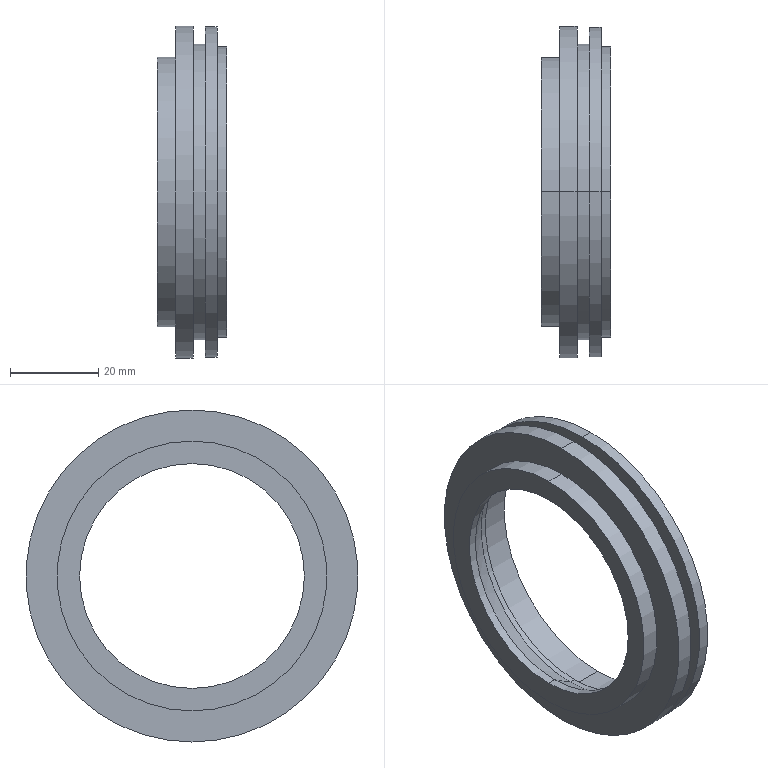Part | STEP file | Dust ring 1 | 1 solid | 25 faces | box 15.692 x 75.322 x 75.322 mm | volume 18737 mm3 | cylinder 16 | plane 7 | cone 2 | commonest cylinder face diameters 50.999 x2 57.197 x2 60.022 x2 61.199 x2 65.906 x2 67.083 x2
STEP:
#1=CARTESIAN_POINT('',(19.871,0.,37.661));
#2=VERTEX_POINT('',#1);
#3=CARTESIAN_POINT('',(19.871,0.,-37.661));
#4=VERTEX_POINT('',#3);
#5=CARTESIAN_POINT('',(19.871,0.,0.));
#6=DIRECTION('',(-1.,0.,0.));
#7=DIRECTION('',(0.,0.,1.));
#8=AXIS2_PLACEMENT_3D('',#5,#6,#7);
#9=CIRCLE('',#8,37.661);
#10=EDGE_CURVE('',#2,#4,#9,.T.);
#11=ORIENTED_EDGE('',*,*,#10,.T.);
#12=CARTESIAN_POINT('',(15.948,0.,-37.661));
#13=VERTEX_POINT('',#12);
#14=CARTESIAN_POINT('',(-10.442,0.,-37.661));
#15=DIRECTION('',(-1.,0.,0.));
#16=VECTOR('',#15,1000.);
#17=LINE('',#14,#16);
#18=EDGE_CURVE('',#4,#13,#17,.T.);
#19=ORIENTED_EDGE('',*,*,#18,.T.);
#20=CARTESIAN_POINT('',(15.948,0.,37.661));
#21=VERTEX_POINT('',#20);
#22=CARTESIAN_POINT('',(15.948,0.,0.));
#23=DIRECTION('',(-1.,0.,0.));
#24=DIRECTION('',(0.,0.,1.));
#25=AXIS2_PLACEMENT_3D('',#22,#23,#24);
#26=CIRCLE('',#25,37.661);
#27=EDGE_CURVE('',#21,#13,#26,.T.);
#28=ORIENTED_EDGE('',*,*,#27,.F.);
#29=CARTESIAN_POINT('',(-10.442,0.,37.661));
#30=DIRECTION('',(-1.,0.,0.));
#31=VECTOR('',#30,1000.);
#32=LINE('',#29,#31);
#33=EDGE_CURVE('',#2,#21,#32,.T.);
#34=ORIENTED_EDGE('',*,*,#33,.F.);
#35=EDGE_LOOP('',(#11,#19,#28,#34));
#36=FACE_OUTER_BOUND('',#35,.T.);
#37=CARTESIAN_POINT('',(-10.442,0.,0.));
#38=DIRECTION('',(-1.,0.,0.));
#39=DIRECTION('',(0.,0.,1.));
#40=AXIS2_PLACEMENT_3D('',#37,#38,#39);
#41=CYLINDRICAL_SURFACE('',#40,37.661);
#42=ADVANCED_FACE('',(#36),#41,.T.);
#43=CARTESIAN_POINT('',(22.696,0.,33.542));
#44=VERTEX_POINT('',#43);
#45=CARTESIAN_POINT('',(22.696,0.,-33.542));
#46=VERTEX_POINT('',#45);
#47=CARTESIAN_POINT('',(22.696,0.,0.));
#48=DIRECTION('',(-1.,0.,0.));
#49=DIRECTION('',(0.,0.,1.));
#50=AXIS2_PLACEMENT_3D('',#47,#48,#49);
#51=CIRCLE('',#50,33.542);
#52=EDGE_CURVE('',#44,#46,#51,.T.);
#53=ORIENTED_EDGE('',*,*,#52,.T.);
#54=CARTESIAN_POINT('',(19.871,0.,-33.542));
#55=VERTEX_POINT('',#54);
#56=CARTESIAN_POINT('',(-10.442,0.,-33.542));
#57=DIRECTION('',(-1.,0.,0.));
#58=VECTOR('',#57,1000.);
#59=LINE('',#56,#58);
#60=EDGE_CURVE('',#46,#55,#59,.T.);
#61=ORIENTED_EDGE('',*,*,#60,.T.);
#62=CARTESIAN_POINT('',(19.871,0.,33.542));
#63=VERTEX_POINT('',#62);
#64=CARTESIAN_POINT('',(19.871,0.,0.));
#65=DIRECTION('',(-1.,0.,0.));
#66=DIRECTION('',(0.,0.,1.));
#67=AXIS2_PLACEMENT_3D('',#64,#65,#66);
#68=CIRCLE('',#67,33.542);
#69=EDGE_CURVE('',#63,#55,#68,.T.);
#70=ORIENTED_EDGE('',*,*,#69,.F.);
#71=CARTESIAN_POINT('',(-10.442,0.,33.542));
#72=DIRECTION('',(-1.,0.,0.));
#73=VECTOR('',#72,1000.);
#74=LINE('',#71,#73);
#75=EDGE_CURVE('',#44,#63,#74,.T.);
#76=ORIENTED_EDGE('',*,*,#75,.F.);
#77=EDGE_LOOP('',(#53,#61,#70,#76));
#78=FACE_OUTER_BOUND('',#77,.T.);
#79=CARTESIAN_POINT('',(-10.442,0.,0.));
#80=DIRECTION('',(-1.,0.,0.));
#81=DIRECTION('',(0.,0.,1.));
#82=AXIS2_PLACEMENT_3D('',#79,#80,#81);
#83=CYLINDRICAL_SURFACE('',#82,33.542);
#84=ADVANCED_FACE('',(#78),#83,.T.);
#85=CARTESIAN_POINT('',(25.324,0.,37.465));
#86=VERTEX_POINT('',#85);
#87=CARTESIAN_POINT('',(25.324,0.,-37.465));
#88=VERTEX_POINT('',#87);
#89=CARTESIAN_POINT('',(25.324,0.,0.));
#90=DIRECTION('',(-1.,0.,0.));
#91=DIRECTION('',(0.,0.,1.));
#92=AXIS2_PLACEMENT_3D('',#89,#90,#91);
#93=CIRCLE('',#92,37.465);
#94=EDGE_CURVE('',#86,#88,#93,.T.);
#95=ORIENTED_EDGE('',*,*,#94,.T.);
#96=CARTESIAN_POINT('',(22.696,0.,-37.465));
#97=VERTEX_POINT('',#96);
#98=CARTESIAN_POINT('',(-10.442,0.,-37.465));
#99=DIRECTION('',(-1.,0.,0.));
#100=VECTOR('',#99,1000.);
#101=LINE('',#98,#100);
#102=EDGE_CURVE('',#88,#97,#101,.T.);
#103=ORIENTED_EDGE('',*,*,#102,.T.);
#104=CARTESIAN_POINT('',(22.696,0.,37.465));
#105=VERTEX_POINT('',#104);
#106=CARTESIAN_POINT('',(22.696,0.,0.));
#107=DIRECTION('',(-1.,0.,0.));
#108=DIRECTION('',(0.,0.,1.));
#109=AXIS2_PLACEMENT_3D('',#106,#107,#108);
#110=CIRCLE('',#109,37.465);
#111=EDGE_CURVE('',#105,#97,#110,.T.);
#112=ORIENTED_EDGE('',*,*,#111,.F.);
#113=CARTESIAN_POINT('',(-10.442,0.,37.465));
#114=DIRECTION('',(-1.,0.,0.));
#115=VECTOR('',#114,1000.);
#116=LINE('',#113,#115);
#117=EDGE_CURVE('',#86,#105,#116,.T.);
#118=ORIENTED_EDGE('',*,*,#117,.F.);
#119=EDGE_LOOP('',(#95,#103,#112,#118));
#120=FACE_OUTER_BOUND('',#119,.T.);
#121=CARTESIAN_POINT('',(-10.442,0.,0.));
#122=DIRECTION('',(-1.,0.,0.));
#123=DIRECTION('',(0.,0.,1.));
#124=AXIS2_PLACEMENT_3D('',#121,#122,#123);
#125=CYLINDRICAL_SURFACE('',#124,37.465);
#126=ADVANCED_FACE('',(#120),#125,.T.);
#127=CARTESIAN_POINT('',(27.482,0.,32.953));
#128=VERTEX_POINT('',#127);
#129=CARTESIAN_POINT('',(27.482,0.,-32.953));
#130=VERTEX_POINT('',#129);
#131=CARTESIAN_POINT('',(27.482,0.,0.));
#132=DIRECTION('',(-1.,0.,0.));
#133=DIRECTION('',(0.,0.,1.));
#134=AXIS2_PLACEMENT_3D('',#131,#132,#133);
#135=CIRCLE('',#134,32.953);
#136=EDGE_CURVE('',#128,#130,#135,.T.);
#137=ORIENTED_EDGE('',*,*,#136,.T.);
#138=CARTESIAN_POINT('',(25.324,0.,-32.953));
#139=VERTEX_POINT('',#138);
#140=CARTESIAN_POINT('',(-10.442,0.,-32.953));
#141=DIRECTION('',(-1.,0.,0.));
#142=VECTOR('',#141,1000.);
#143=LINE('',#140,#142);
#144=EDGE_CURVE('',#130,#139,#143,.T.);
#145=ORIENTED_EDGE('',*,*,#144,.T.);
#146=CARTESIAN_POINT('',(25.324,0.,32.953));
#147=VERTEX_POINT('',#146);
#148=CARTESIAN_POINT('',(25.324,0.,0.));
#149=DIRECTION('',(-1.,0.,0.));
#150=DIRECTION('',(0.,0.,1.));
#151=AXIS2_PLACEMENT_3D('',#148,#149,#150);
#152=CIRCLE('',#151,32.953);
#153=EDGE_CURVE('',#147,#139,#152,.T.);
#154=ORIENTED_EDGE('',*,*,#153,.F.);
#155=CARTESIAN_POINT('',(-10.442,0.,32.953));
#156=DIRECTION('',(-1.,0.,0.));
#157=VECTOR('',#156,1000.);
#158=LINE('',#155,#157);
#159=EDGE_CURVE('',#128,#147,#158,.T.);
#160=ORIENTED_EDGE('',*,*,#159,.F.);
#161=EDGE_LOOP('',(#137,#145,#154,#160));
#162=FACE_OUTER_BOUND('',#161,.T.);
#163=CARTESIAN_POINT('',(-10.442,0.,0.));
#164=DIRECTION('',(-1.,0.,0.));
#165=DIRECTION('',(0.,0.,1.));
#166=AXIS2_PLACEMENT_3D('',#163,#164,#165);
#167=CYLINDRICAL_SURFACE('',#166,32.953);
#168=ADVANCED_FACE('',(#162),#167,.T.);
#169=CARTESIAN_POINT('',(27.482,0.,-30.011));
#170=VERTEX_POINT('',#169);
#171=CARTESIAN_POINT('',(27.482,0.,30.011));
#172=VERTEX_POINT('',#171);
#173=CARTESIAN_POINT('',(27.482,0.,0.));
#174=DIRECTION('',(-1.,0.,0.));
#175=DIRECTION('',(0.,0.,1.));
#176=AXIS2_PLACEMENT_3D('',#173,#174,#175);
#177=CIRCLE('',#176,30.011);
#178=EDGE_CURVE('',#170,#172,#177,.T.);
#179=ORIENTED_EDGE('',*,*,#178,.F.);
#180=CARTESIAN_POINT('',(20.028,0.,-30.011));
#181=VERTEX_POINT('',#180);
#182=CARTESIAN_POINT('',(-10.442,0.,-30.011));
#183=DIRECTION('',(-1.,0.,0.));
#184=VECTOR('',#183,1000.);
#185=LINE('',#182,#184);
#186=EDGE_CURVE('',#170,#181,#185,.T.);
#187=ORIENTED_EDGE('',*,*,#186,.T.);
#188=CARTESIAN_POINT('',(20.028,0.,30.011));
#189=VERTEX_POINT('',#188);
#190=CARTESIAN_POINT('',(20.028,0.,0.));
#191=DIRECTION('',(-1.,0.,0.));
#192=DIRECTION('',(0.,0.,1.));
#193=AXIS2_PLACEMENT_3D('',#190,#191,#192);
#194=CIRCLE('',#193,30.011);
#195=EDGE_CURVE('',#181,#189,#194,.T.);
#196=ORIENTED_EDGE('',*,*,#195,.T.);
#197=CARTESIAN_POINT('',(-10.442,0.,30.011));
#198=DIRECTION('',(-1.,0.,0.));
#199=VECTOR('',#198,1000.);
#200=LINE('',#197,#199);
#201=EDGE_CURVE('',#172,#189,#200,.T.);
#202=ORIENTED_EDGE('',*,*,#201,.F.);
#203=EDGE_LOOP('',(#179,#187,#196,#202));
#204=FACE_OUTER_BOUND('',#203,.T.);
#205=CARTESIAN_POINT('',(-10.442,0.,0.));
#206=DIRECTION('',(-1.,0.,0.));
#207=DIRECTION('',(0.,0.,1.));
#208=AXIS2_PLACEMENT_3D('',#205,#206,#207);
#209=CYLINDRICAL_SURFACE('',#208,30.011);
#210=ADVANCED_FACE('',(#204),#209,.F.);
#211=CARTESIAN_POINT('',(20.028,0.,-28.599));
#212=VERTEX_POINT('',#211);
#213=CARTESIAN_POINT('',(20.028,0.,28.599));
#214=VERTEX_POINT('',#213);
#215=CARTESIAN_POINT('',(20.028,0.,0.));
#216=DIRECTION('',(-1.,0.,0.));
#217=DIRECTION('',(0.,0.,1.));
#218=AXIS2_PLACEMENT_3D('',#215,#216,#217);
#219=CIRCLE('',#218,28.599);
#220=EDGE_CURVE('',#212,#214,#219,.T.);
#221=ORIENTED_EDGE('',*,*,#220,.F.);
#222=CARTESIAN_POINT('',(18.655,0.,-28.599));
#223=VERTEX_POINT('',#222);
#224=CARTESIAN_POINT('',(-10.442,0.,-28.599));
#225=DIRECTION('',(-1.,0.,0.));
#226=VECTOR('',#225,1000.);
#227=LINE('',#224,#226);
#228=EDGE_CURVE('',#212,#223,#227,.T.);
#229=ORIENTED_EDGE('',*,*,#228,.T.);
#230=CARTESIAN_POINT('',(18.655,0.,28.599));
#231=VERTEX_POINT('',#230);
#232=CARTESIAN_POINT('',(18.655,0.,0.));
#233=DIRECTION('',(-1.,0.,0.));
#234=DIRECTION('',(0.,0.,1.));
#235=AXIS2_PLACEMENT_3D('',#232,#233,#234);
#236=CIRCLE('',#235,28.599);
#237=EDGE_CURVE('',#223,#231,#236,.T.);
#238=ORIENTED_EDGE('',*,*,#237,.T.);
#239=CARTESIAN_POINT('',(-10.442,0.,28.599));
#240=DIRECTION('',(-1.,0.,0.));
#241=VECTOR('',#240,1000.);
#242=LINE('',#239,#241);
#243=EDGE_CURVE('',#214,#231,#242,.T.);
#244=ORIENTED_EDGE('',*,*,#243,.F.);
#245=EDGE_LOOP('',(#221,#229,#238,#244));
#246=FACE_OUTER_BOUND('',#245,.T.);
#247=CARTESIAN_POINT('',(-10.442,0.,0.));
#248=DIRECTION('',(-1.,0.,0.));
#249=DIRECTION('',(0.,0.,1.));
#250=AXIS2_PLACEMENT_3D('',#247,#248,#249);
#251=CYLINDRICAL_SURFACE('',#250,28.599);
#252=ADVANCED_FACE('',(#246),#251,.F.);
#253=CARTESIAN_POINT('',(13.751,0.,-25.5));
#254=VERTEX_POINT('',#253);
#255=CARTESIAN_POINT('',(13.751,0.,25.5));
#256=VERTEX_POINT('',#255);
#257=CARTESIAN_POINT('',(13.751,0.,0.));
#258=DIRECTION('',(-1.,0.,0.));
#259=DIRECTION('',(0.,0.,1.));
#260=AXIS2_PLACEMENT_3D('',#257,#258,#259);
#261=CIRCLE('',#260,25.5);
#262=EDGE_CURVE('',#254,#256,#261,.T.);
#263=ORIENTED_EDGE('',*,*,#262,.T.);
#264=CARTESIAN_POINT('',(13.751,0.,25.5));
#265=DIRECTION('',(0.8453,0.,0.5342));
#266=VECTOR('',#265,1000.);
#267=LINE('',#264,#266);
#268=EDGE_CURVE('',#256,#231,#267,.T.);
#269=ORIENTED_EDGE('',*,*,#268,.T.);
#270=ORIENTED_EDGE('',*,*,#237,.F.);
#271=CARTESIAN_POINT('',(13.751,0.,-25.5));
#272=DIRECTION('',(0.8453,0.,-0.5342));
#273=VECTOR('',#272,1000.);
#274=LINE('',#271,#273);
#275=EDGE_CURVE('',#254,#223,#274,.T.);
#276=ORIENTED_EDGE('',*,*,#275,.F.);
#277=EDGE_LOOP('',(#263,#269,#270,#276));
#278=FACE_OUTER_BOUND('',#277,.T.);
#279=CARTESIAN_POINT('',(13.751,0.,0.));
#280=DIRECTION('',(1.,0.,0.));
#281=DIRECTION('',(0.,0.,-1.));
#282=AXIS2_PLACEMENT_3D('',#279,#280,#281);
#283=CONICAL_SURFACE('',#282,25.5,0.5636);
#284=ADVANCED_FACE('',(#278),#283,.F.);
#285=ORIENTED_EDGE('',*,*,#262,.F.);
#286=CARTESIAN_POINT('',(11.79,0.,-25.5));
#287=VERTEX_POINT('',#286);
#288=CARTESIAN_POINT('',(-10.442,0.,-25.5));
#289=DIRECTION('',(-1.,0.,0.));
#290=VECTOR('',#289,1000.);
#291=LINE('',#288,#290);
#292=EDGE_CURVE('',#254,#287,#291,.T.);
#293=ORIENTED_EDGE('',*,*,#292,.T.);
#294=CARTESIAN_POINT('',(11.79,0.,25.5));
#295=VERTEX_POINT('',#294);
#296=CARTESIAN_POINT('',(11.79,0.,0.));
#297=DIRECTION('',(-1.,0.,0.));
#298=DIRECTION('',(0.,0.,1.));
#299=AXIS2_PLACEMENT_3D('',#296,#297,#298);
#300=CIRCLE('',#299,25.5);
#301=EDGE_CURVE('',#287,#295,#300,.T.);
#302=ORIENTED_EDGE('',*,*,#301,.T.);
#303=CARTESIAN_POINT('',(-10.442,0.,25.5));
#304=DIRECTION('',(-1.,0.,0.));
#305=VECTOR('',#304,1000.);
#306=LINE('',#303,#305);
#307=EDGE_CURVE('',#256,#295,#306,.T.);
#308=ORIENTED_EDGE('',*,*,#307,.F.);
#309=EDGE_LOOP('',(#285,#293,#302,#308));
#310=FACE_OUTER_BOUND('',#309,.T.);
#311=CARTESIAN_POINT('',(-10.442,0.,0.));
#312=DIRECTION('',(-1.,0.,0.));
#313=DIRECTION('',(0.,0.,1.));
#314=AXIS2_PLACEMENT_3D('',#311,#312,#313);
#315=CYLINDRICAL_SURFACE('',#314,25.5);
#316=ADVANCED_FACE('',(#310),#315,.F.);
#317=CARTESIAN_POINT('',(15.948,0.,30.599));
#318=VERTEX_POINT('',#317);
#319=CARTESIAN_POINT('',(15.948,0.,-30.599));
#320=VERTEX_POINT('',#319);
#321=CARTESIAN_POINT('',(15.948,0.,0.));
#322=DIRECTION('',(-1.,0.,0.));
#323=DIRECTION('',(0.,0.,1.));
#324=AXIS2_PLACEMENT_3D('',#321,#322,#323);
#325=CIRCLE('',#324,30.599);
#326=EDGE_CURVE('',#318,#320,#325,.T.);
#327=ORIENTED_EDGE('',*,*,#326,.T.);
#328=CARTESIAN_POINT('',(11.79,0.,-30.599));
#329=VERTEX_POINT('',#328);
#330=CARTESIAN_POINT('',(-10.442,0.,-30.599));
#331=DIRECTION('',(-1.,0.,0.));
#332=VECTOR('',#331,1000.);
#333=LINE('',#330,#332);
#334=EDGE_CURVE('',#320,#329,#333,.T.);
#335=ORIENTED_EDGE('',*,*,#334,.T.);
#336=CARTESIAN_POINT('',(11.79,0.,30.599));
#337=VERTEX_POINT('',#336);
#338=CARTESIAN_POINT('',(11.79,0.,0.));
#339=DIRECTION('',(-1.,0.,0.));
#340=DIRECTION('',(0.,0.,1.));
#341=AXIS2_PLACEMENT_3D('',#338,#339,#340);
#342=CIRCLE('',#341,30.599);
#343=EDGE_CURVE('',#337,#329,#342,.T.);
#344=ORIENTED_EDGE('',*,*,#343,.F.);
#345=CARTESIAN_POINT('',(-10.442,0.,30.599));
#346=DIRECTION('',(-1.,0.,0.));
#347=VECTOR('',#346,1000.);
#348=LINE('',#345,#347);
#349=EDGE_CURVE('',#318,#337,#348,.T.);
#350=ORIENTED_EDGE('',*,*,#349,.F.);
#351=EDGE_LOOP('',(#327,#335,#344,#350));
#352=FACE_OUTER_BOUND('',#351,.T.);
#353=CARTESIAN_POINT('',(-10.442,0.,0.));
#354=DIRECTION('',(-1.,0.,0.));
#355=DIRECTION('',(0.,0.,1.));
#356=AXIS2_PLACEMENT_3D('',#353,#354,#355);
#357=CYLINDRICAL_SURFACE('',#356,30.599);
#358=ADVANCED_FACE('',(#352),#357,.T.);
#359=ORIENTED_EDGE('',*,*,#334,.F.);
#360=CARTESIAN_POINT('',(15.948,0.,0.));
#361=DIRECTION('',(-1.,0.,0.));
#362=DIRECTION('',(0.,0.,1.));
#363=AXIS2_PLACEMENT_3D('',#360,#361,#362);
#364=CIRCLE('',#363,30.599);
#365=EDGE_CURVE('',#320,#318,#364,.T.);
#366=ORIENTED_EDGE('',*,*,#365,.T.);
#367=ORIENTED_EDGE('',*,*,#349,.T.);
#368=CARTESIAN_POINT('',(11.79,0.,0.));
#369=DIRECTION('',(-1.,0.,0.));
#370=DIRECTION('',(0.,0.,1.));
#371=AXIS2_PLACEMENT_3D('',#368,#369,#370);
#372=CIRCLE('',#371,30.599);
#373=EDGE_CURVE('',#329,#337,#372,.T.);
#374=ORIENTED_EDGE('',*,*,#373,.F.);
#375=EDGE_LOOP('',(#359,#366,#367,#374));
#376=FACE_OUTER_BOUND('',#375,.T.);
#377=CARTESIAN_POINT('',(-10.442,0.,0.));
#378=DIRECTION('',(-1.,0.,0.));
#379=DIRECTION('',(0.,0.,1.));
#380=AXIS2_PLACEMENT_3D('',#377,#378,#379);
#381=CYLINDRICAL_SURFACE('',#380,30.599);
#382=ADVANCED_FACE('',(#376),#381,.T.);
#383=ORIENTED_EDGE('',*,*,#343,.T.);
#384=ORIENTED_EDGE('',*,*,#373,.T.);
#385=EDGE_LOOP('',(#383,#384));
#386=FACE_OUTER_BOUND('',#385,.T.);
#387=CARTESIAN_POINT('',(11.79,0.,0.));
#388=DIRECTION('',(-1.,0.,0.));
#389=DIRECTION('',(0.,0.,1.));
#390=AXIS2_PLACEMENT_3D('',#387,#388,#389);
#391=CIRCLE('',#390,25.5);
#392=EDGE_CURVE('',#295,#287,#391,.T.);
#393=ORIENTED_EDGE('',*,*,#392,.F.);
#394=ORIENTED_EDGE('',*,*,#301,.F.);
#395=EDGE_LOOP('',(#393,#394));
#396=FACE_BOUND('',#395,.T.);
#397=CARTESIAN_POINT('',(11.79,0.,0.));
#398=DIRECTION('',(-1.,0.,0.));
#399=DIRECTION('',(0.,0.,1.));
#400=AXIS2_PLACEMENT_3D('',#397,#398,#399);
#401=PLANE('',#400);
#402=ADVANCED_FACE('',(#386,#396),#401,.T.);
#403=ORIENTED_EDGE('',*,*,#292,.F.);
#404=CARTESIAN_POINT('',(13.751,0.,0.));
#405=DIRECTION('',(-1.,0.,0.));
#406=DIRECTION('',(0.,0.,1.));
#407=AXIS2_PLACEMENT_3D('',#404,#405,#406);
#408=CIRCLE('',#407,25.5);
#409=EDGE_CURVE('',#256,#254,#408,.T.);
#410=ORIENTED_EDGE('',*,*,#409,.F.);
#411=ORIENTED_EDGE('',*,*,#307,.T.);
#412=ORIENTED_EDGE('',*,*,#392,.T.);
#413=EDGE_LOOP('',(#403,#410,#411,#412));
#414=FACE_OUTER_BOUND('',#413,.T.);
#415=CARTESIAN_POINT('',(-10.442,0.,0.));
#416=DIRECTION('',(-1.,0.,0.));
#417=DIRECTION('',(0.,0.,1.));
#418=AXIS2_PLACEMENT_3D('',#415,#416,#417);
#419=CYLINDRICAL_SURFACE('',#418,25.5);
#420=ADVANCED_FACE('',(#414),#419,.F.);
#421=ORIENTED_EDGE('',*,*,#268,.F.);
#422=ORIENTED_EDGE('',*,*,#409,.T.);
#423=ORIENTED_EDGE('',*,*,#275,.T.);
#424=CARTESIAN_POINT('',(18.655,0.,0.));
#425=DIRECTION('',(-1.,0.,0.));
#426=DIRECTION('',(0.,0.,1.));
#427=AXIS2_PLACEMENT_3D('',#424,#425,#426);
#428=CIRCLE('',#427,28.599);
#429=EDGE_CURVE('',#231,#223,#428,.T.);
#430=ORIENTED_EDGE('',*,*,#429,.F.);
#431=EDGE_LOOP('',(#421,#422,#423,#430));
#432=FACE_OUTER_BOUND('',#431,.T.);
#433=CARTESIAN_POINT('',(13.751,0.,0.));
#434=DIRECTION('',(1.,0.,0.));
#435=DIRECTION('',(0.,0.,-1.));
#436=AXIS2_PLACEMENT_3D('',#433,#434,#435);
#437=CONICAL_SURFACE('',#436,25.5,0.5636);
#438=ADVANCED_FACE('',(#432),#437,.F.);
#439=ORIENTED_EDGE('',*,*,#228,.F.);
#440=CARTESIAN_POINT('',(20.028,0.,0.));
#441=DIRECTION('',(-1.,0.,0.));
#442=DIRECTION('',(0.,0.,1.));
#443=AXIS2_PLACEMENT_3D('',#440,#441,#442);
#444=CIRCLE('',#443,28.599);
#445=EDGE_CURVE('',#214,#212,#444,.T.);
#446=ORIENTED_EDGE('',*,*,#445,.F.);
#447=ORIENTED_EDGE('',*,*,#243,.T.);
#448=ORIENTED_EDGE('',*,*,#429,.T.);
#449=EDGE_LOOP('',(#439,#446,#447,#448));
#450=FACE_OUTER_BOUND('',#449,.T.);
#451=CARTESIAN_POINT('',(-10.442,0.,0.));
#452=DIRECTION('',(-1.,0.,0.));
#453=DIRECTION('',(0.,0.,1.));
#454=AXIS2_PLACEMENT_3D('',#451,#452,#453);
#455=CYLINDRICAL_SURFACE('',#454,28.599);
#456=ADVANCED_FACE('',(#450),#455,.F.);
#457=ORIENTED_EDGE('',*,*,#445,.T.);
#458=ORIENTED_EDGE('',*,*,#220,.T.);
#459=EDGE_LOOP('',(#457,#458));
#460=FACE_BOUND('',#459,.T.);
#461=CARTESIAN_POINT('',(20.028,0.,0.));
#462=DIRECTION('',(-1.,0.,0.));
#463=DIRECTION('',(0.,0.,1.));
#464=AXIS2_PLACEMENT_3D('',#461,#462,#463);
#465=CIRCLE('',#464,30.011);
#466=EDGE_CURVE('',#189,#181,#465,.T.);
#467=ORIENTED_EDGE('',*,*,#466,.F.);
#468=ORIENTED_EDGE('',*,*,#195,.F.);
#469=EDGE_LOOP('',(#467,#468));
#470=FACE_OUTER_BOUND('',#469,.T.);
#471=CARTESIAN_POINT('',(20.028,0.,0.));
#472=DIRECTION('',(1.,0.,0.));
#473=DIRECTION('',(0.,0.,-1.));
#474=AXIS2_PLACEMENT_3D('',#471,#472,#473);
#475=PLANE('',#474);
#476=ADVANCED_FACE('',(#460,#470),#475,.T.);
#477=ORIENTED_EDGE('',*,*,#186,.F.);
#478=CARTESIAN_POINT('',(27.482,0.,0.));
#479=DIRECTION('',(-1.,0.,0.));
#480=DIRECTION('',(0.,0.,1.));
#481=AXIS2_PLACEMENT_3D('',#478,#479,#480);
#482=CIRCLE('',#481,30.011);
#483=EDGE_CURVE('',#172,#170,#482,.T.);
#484=ORIENTED_EDGE('',*,*,#483,.F.);
#485=ORIENTED_EDGE('',*,*,#201,.T.);
#486=ORIENTED_EDGE('',*,*,#466,.T.);
#487=EDGE_LOOP('',(#477,#484,#485,#486));
#488=FACE_OUTER_BOUND('',#487,.T.);
#489=CARTESIAN_POINT('',(-10.442,0.,0.));
#490=DIRECTION('',(-1.,0.,0.));
#491=DIRECTION('',(0.,0.,1.));
#492=AXIS2_PLACEMENT_3D('',#489,#490,#491);
#493=CYLINDRICAL_SURFACE('',#492,30.011);
#494=ADVANCED_FACE('',(#488),#493,.F.);
#495=ORIENTED_EDGE('',*,*,#136,.F.);
#496=CARTESIAN_POINT('',(27.482,0.,0.));
#497=DIRECTION('',(-1.,0.,0.));
#498=DIRECTION('',(0.,0.,1.));
#499=AXIS2_PLACEMENT_3D('',#496,#497,#498);
#500=CIRCLE('',#499,32.953);
#501=EDGE_CURVE('',#130,#128,#500,.T.);
#502=ORIENTED_EDGE('',*,*,#501,.F.);
#503=EDGE_LOOP('',(#495,#502));
#504=FACE_OUTER_BOUND('',#503,.T.);
#505=ORIENTED_EDGE('',*,*,#483,.T.);
#506=ORIENTED_EDGE('',*,*,#178,.T.);
#507=EDGE_LOOP('',(#505,#506));
#508=FACE_BOUND('',#507,.T.);
#509=CARTESIAN_POINT('',(27.482,0.,0.));
#510=DIRECTION('',(-1.,0.,0.));
#511=DIRECTION('',(0.,0.,1.));
#512=AXIS2_PLACEMENT_3D('',#509,#510,#511);
#513=PLANE('',#512);
#514=ADVANCED_FACE('',(#504,#508),#513,.F.);
#515=ORIENTED_EDGE('',*,*,#144,.F.);
#516=ORIENTED_EDGE('',*,*,#501,.T.);
#517=ORIENTED_EDGE('',*,*,#159,.T.);
#518=CARTESIAN_POINT('',(25.324,0.,0.));
#519=DIRECTION('',(-1.,0.,0.));
#520=DIRECTION('',(0.,0.,1.));
#521=AXIS2_PLACEMENT_3D('',#518,#519,#520);
#522=CIRCLE('',#521,32.953);
#523=EDGE_CURVE('',#139,#147,#522,.T.);
#524=ORIENTED_EDGE('',*,*,#523,.F.);
#525=EDGE_LOOP('',(#515,#516,#517,#524));
#526=FACE_OUTER_BOUND('',#525,.T.);
#527=CARTESIAN_POINT('',(-10.442,0.,0.));
#528=DIRECTION('',(-1.,0.,0.));
#529=DIRECTION('',(0.,0.,1.));
#530=AXIS2_PLACEMENT_3D('',#527,#528,#529);
#531=CYLINDRICAL_SURFACE('',#530,32.953);
#532=ADVANCED_FACE('',(#526),#531,.T.);
#533=ORIENTED_EDGE('',*,*,#94,.F.);
#534=CARTESIAN_POINT('',(25.324,0.,0.));
#535=DIRECTION('',(-1.,0.,0.));
#536=DIRECTION('',(0.,0.,1.));
#537=AXIS2_PLACEMENT_3D('',#534,#535,#536);
#538=CIRCLE('',#537,37.465);
#539=EDGE_CURVE('',#88,#86,#538,.T.);
#540=ORIENTED_EDGE('',*,*,#539,.F.);
#541=EDGE_LOOP('',(#533,#540));
#542=FACE_OUTER_BOUND('',#541,.T.);
#543=ORIENTED_EDGE('',*,*,#153,.T.);
#544=ORIENTED_EDGE('',*,*,#523,.T.);
#545=EDGE_LOOP('',(#543,#544));
#546=FACE_BOUND('',#545,.T.);
#547=CARTESIAN_POINT('',(25.324,0.,0.));
#548=DIRECTION('',(-1.,0.,0.));
#549=DIRECTION('',(0.,0.,1.));
#550=AXIS2_PLACEMENT_3D('',#547,#548,#549);
#551=PLANE('',#550);
#552=ADVANCED_FACE('',(#542,#546),#551,.F.);
#553=ORIENTED_EDGE('',*,*,#102,.F.);
#554=ORIENTED_EDGE('',*,*,#539,.T.);
#555=ORIENTED_EDGE('',*,*,#117,.T.);
#556=CARTESIAN_POINT('',(22.696,0.,0.));
#557=DIRECTION('',(-1.,0.,0.));
#558=DIRECTION('',(0.,0.,1.));
#559=AXIS2_PLACEMENT_3D('',#556,#557,#558);
#560=CIRCLE('',#559,37.465);
#561=EDGE_CURVE('',#97,#105,#560,.T.);
#562=ORIENTED_EDGE('',*,*,#561,.F.);
#563=EDGE_LOOP('',(#553,#554,#555,#562));
#564=FACE_OUTER_BOUND('',#563,.T.);
#565=CARTESIAN_POINT('',(-10.442,0.,0.));
#566=DIRECTION('',(-1.,0.,0.));
#567=DIRECTION('',(0.,0.,1.));
#568=AXIS2_PLACEMENT_3D('',#565,#566,#567);
#569=CYLINDRICAL_SURFACE('',#568,37.465);
#570=ADVANCED_FACE('',(#564),#569,.T.);
#571=ORIENTED_EDGE('',*,*,#52,.F.);
#572=CARTESIAN_POINT('',(22.696,0.,0.));
#573=DIRECTION('',(-1.,0.,0.));
#574=DIRECTION('',(0.,0.,1.));
#575=AXIS2_PLACEMENT_3D('',#572,#573,#574);
#576=CIRCLE('',#575,33.542);
#577=EDGE_CURVE('',#46,#44,#576,.T.);
#578=ORIENTED_EDGE('',*,*,#577,.F.);
#579=EDGE_LOOP('',(#571,#578));
#580=FACE_BOUND('',#579,.T.);
#581=ORIENTED_EDGE('',*,*,#111,.T.);
#582=ORIENTED_EDGE('',*,*,#561,.T.);
#583=EDGE_LOOP('',(#581,#582));
#584=FACE_OUTER_BOUND('',#583,.T.);
#585=CARTESIAN_POINT('',(22.696,0.,0.));
#586=DIRECTION('',(1.,0.,0.));
#587=DIRECTION('',(0.,0.,-1.));
#588=AXIS2_PLACEMENT_3D('',#585,#586,#587);
#589=PLANE('',#588);
#590=ADVANCED_FACE('',(#580,#584),#589,.F.);
#591=ORIENTED_EDGE('',*,*,#60,.F.);
#592=ORIENTED_EDGE('',*,*,#577,.T.);
#593=ORIENTED_EDGE('',*,*,#75,.T.);
#594=CARTESIAN_POINT('',(19.871,0.,0.));
#595=DIRECTION('',(-1.,0.,0.));
#596=DIRECTION('',(0.,0.,1.));
#597=AXIS2_PLACEMENT_3D('',#594,#595,#596);
#598=CIRCLE('',#597,33.542);
#599=EDGE_CURVE('',#55,#63,#598,.T.);
#600=ORIENTED_EDGE('',*,*,#599,.F.);
#601=EDGE_LOOP('',(#591,#592,#593,#600));
#602=FACE_OUTER_BOUND('',#601,.T.);
#603=CARTESIAN_POINT('',(-10.442,0.,0.));
#604=DIRECTION('',(-1.,0.,0.));
#605=DIRECTION('',(0.,0.,1.));
#606=AXIS2_PLACEMENT_3D('',#603,#604,#605);
#607=CYLINDRICAL_SURFACE('',#606,33.542);
#608=ADVANCED_FACE('',(#602),#607,.T.);
#609=ORIENTED_EDGE('',*,*,#10,.F.);
#610=CARTESIAN_POINT('',(19.871,0.,0.));
#611=DIRECTION('',(-1.,0.,0.));
#612=DIRECTION('',(0.,0.,1.));
#613=AXIS2_PLACEMENT_3D('',#610,#611,#612);
#614=CIRCLE('',#613,37.661);
#615=EDGE_CURVE('',#4,#2,#614,.T.);
#616=ORIENTED_EDGE('',*,*,#615,.F.);
#617=EDGE_LOOP('',(#609,#616));
#618=FACE_OUTER_BOUND('',#617,.T.);
#619=ORIENTED_EDGE('',*,*,#69,.T.);
#620=ORIENTED_EDGE('',*,*,#599,.T.);
#621=EDGE_LOOP('',(#619,#620));
#622=FACE_BOUND('',#621,.T.);
#623=CARTESIAN_POINT('',(19.871,0.,0.));
#624=DIRECTION('',(-1.,0.,0.));
#625=DIRECTION('',(0.,0.,1.));
#626=AXIS2_PLACEMENT_3D('',#623,#624,#625);
#627=PLANE('',#626);
#628=ADVANCED_FACE('',(#618,#622),#627,.F.);
#629=ORIENTED_EDGE('',*,*,#18,.F.);
#630=ORIENTED_EDGE('',*,*,#615,.T.);
#631=ORIENTED_EDGE('',*,*,#33,.T.);
#632=CARTESIAN_POINT('',(15.948,0.,0.));
#633=DIRECTION('',(-1.,0.,0.));
#634=DIRECTION('',(0.,0.,1.));
#635=AXIS2_PLACEMENT_3D('',#632,#633,#634);
#636=CIRCLE('',#635,37.661);
#637=EDGE_CURVE('',#13,#21,#636,.T.);
#638=ORIENTED_EDGE('',*,*,#637,.F.);
#639=EDGE_LOOP('',(#629,#630,#631,#638));
#640=FACE_OUTER_BOUND('',#639,.T.);
#641=CARTESIAN_POINT('',(-10.442,0.,0.));
#642=DIRECTION('',(-1.,0.,0.));
#643=DIRECTION('',(0.,0.,1.));
#644=AXIS2_PLACEMENT_3D('',#641,#642,#643);
#645=CYLINDRICAL_SURFACE('',#644,37.661);
#646=ADVANCED_FACE('',(#640),#645,.T.);
#647=ORIENTED_EDGE('',*,*,#326,.F.);
#648=ORIENTED_EDGE('',*,*,#365,.F.);
#649=EDGE_LOOP('',(#647,#648));
#650=FACE_BOUND('',#649,.T.);
#651=ORIENTED_EDGE('',*,*,#27,.T.);
#652=ORIENTED_EDGE('',*,*,#637,.T.);
#653=EDGE_LOOP('',(#651,#652));
#654=FACE_OUTER_BOUND('',#653,.T.);
#655=CARTESIAN_POINT('',(15.948,0.,0.));
#656=DIRECTION('',(1.,0.,0.));
#657=DIRECTION('',(0.,0.,-1.));
#658=AXIS2_PLACEMENT_3D('',#655,#656,#657);
#659=PLANE('',#658);
#660=ADVANCED_FACE('',(#650,#654),#659,.F.);
#661=CLOSED_SHELL('',(#42,#84,#126,#168,#210,#252,#284,#316,#358,#382,#402,#420,#438,#456,#476,#494,#514,#532,#552,#570,#590,#608,#628,#646,#660));
#662=MANIFOLD_SOLID_BREP('',#661);
#663=CARTESIAN_POINT('',(0.,0.,0.));
#664=DIRECTION('',(0.,0.,1.));
#665=DIRECTION('',(1.,0.,0.));
#666=AXIS2_PLACEMENT_3D('',#663,#664,#665);
#667=(LENGTH_UNIT()NAMED_UNIT(*)SI_UNIT(.MILLI.,.METRE.));
#668=UNCERTAINTY_MEASURE_WITH_UNIT(LENGTH_MEASURE(0.00001),#667,'','');
#669=(NAMED_UNIT(*)PLANE_ANGLE_UNIT()SI_UNIT($,.RADIAN.));
#670=(NAMED_UNIT(*)SI_UNIT($,.STERADIAN.)SOLID_ANGLE_UNIT());
#671=(GEOMETRIC_REPRESENTATION_CONTEXT(3)GLOBAL_UNCERTAINTY_ASSIGNED_CONTEXT((#668))GLOBAL_UNIT_ASSIGNED_CONTEXT((#667,#669,#670))REPRESENTATION_CONTEXT('',''));
#672=ADVANCED_BREP_SHAPE_REPRESENTATION('',(#662,#666),#671);